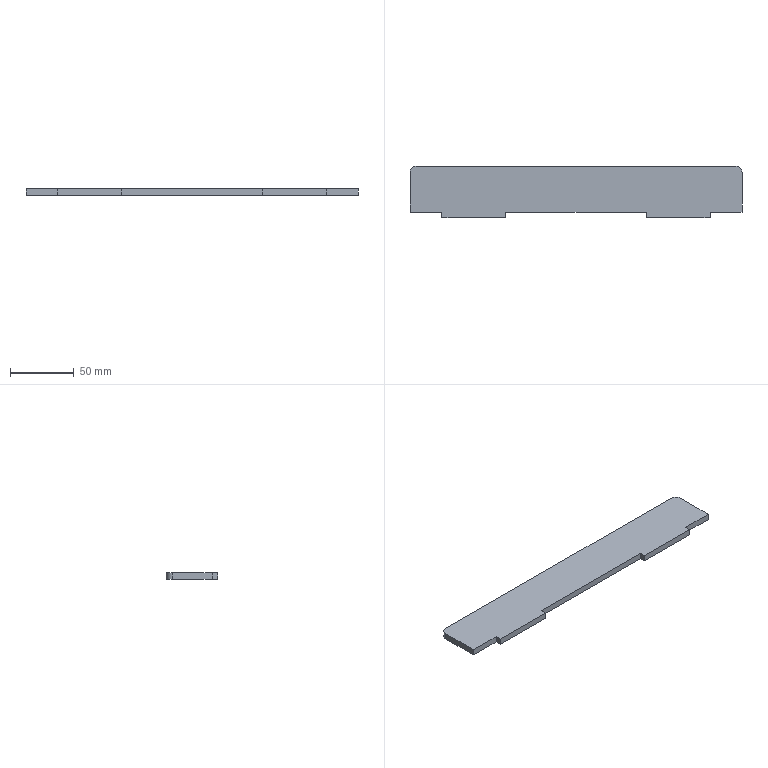Part | SolidWorks | features FlatPattern 1, SMBaseFlange 1, SheetMetal 1 | 1 solid | 16 faces | box 260 x 40.5 x 5 mm | volume 48996 mm3 | plane 14 | cylinder 2 | commonest cylinder face diameters 10 x2
STEP:
#1=CARTESIAN_POINT('',(65.526,-126.05,0.));
#2=VERTEX_POINT('',#1);
#3=CARTESIAN_POINT('',(65.526,-95.05,0.));
#4=VERTEX_POINT('',#3);
#5=CARTESIAN_POINT('',(65.526,-126.05,0.));
#6=DIRECTION('',(0.,1.,0.));
#7=VECTOR('',#6,1000.);
#8=LINE('',#5,#7);
#9=EDGE_CURVE('',#2,#4,#8,.T.);
#10=ORIENTED_EDGE('',*,*,#9,.F.);
#11=CARTESIAN_POINT('',(65.526,-126.05,-5.));
#12=VERTEX_POINT('',#11);
#13=CARTESIAN_POINT('',(65.526,-126.05,-5.));
#14=DIRECTION('',(0.,0.,1.));
#15=VECTOR('',#14,1000.);
#16=LINE('',#13,#15);
#17=EDGE_CURVE('',#12,#2,#16,.T.);
#18=ORIENTED_EDGE('',*,*,#17,.F.);
#19=CARTESIAN_POINT('',(65.526,-95.05,-5.));
#20=VERTEX_POINT('',#19);
#21=CARTESIAN_POINT('',(65.526,-126.05,-5.));
#22=DIRECTION('',(0.,1.,0.));
#23=VECTOR('',#22,1000.);
#24=LINE('',#21,#23);
#25=EDGE_CURVE('',#12,#20,#24,.T.);
#26=ORIENTED_EDGE('',*,*,#25,.T.);
#27=CARTESIAN_POINT('',(65.526,-95.05,-5.));
#28=DIRECTION('',(0.,0.,1.));
#29=VECTOR('',#28,1000.);
#30=LINE('',#27,#29);
#31=EDGE_CURVE('',#20,#4,#30,.T.);
#32=ORIENTED_EDGE('',*,*,#31,.T.);
#33=EDGE_LOOP('',(#10,#18,#26,#32));
#34=FACE_OUTER_BOUND('',#33,.T.);
#35=CARTESIAN_POINT('',(65.526,-126.05,-5.));
#36=DIRECTION('',(1.,0.,0.));
#37=DIRECTION('',(0.,0.,-1.));
#38=AXIS2_PLACEMENT_3D('',#35,#36,#37);
#39=PLANE('',#38);
#40=ADVANCED_FACE('',(#34),#39,.T.);
#41=CARTESIAN_POINT('',(40.526,-126.05,0.));
#42=VERTEX_POINT('',#41);
#43=CARTESIAN_POINT('',(65.526,-126.05,0.));
#44=DIRECTION('',(1.,0.,0.));
#45=VECTOR('',#44,1000.);
#46=LINE('',#43,#45);
#47=EDGE_CURVE('',#42,#2,#46,.T.);
#48=ORIENTED_EDGE('',*,*,#47,.F.);
#49=CARTESIAN_POINT('',(40.526,-126.05,-5.));
#50=VERTEX_POINT('',#49);
#51=CARTESIAN_POINT('',(40.526,-126.05,-5.));
#52=DIRECTION('',(0.,0.,1.));
#53=VECTOR('',#52,1000.);
#54=LINE('',#51,#53);
#55=EDGE_CURVE('',#50,#42,#54,.T.);
#56=ORIENTED_EDGE('',*,*,#55,.F.);
#57=CARTESIAN_POINT('',(65.526,-126.05,-5.));
#58=DIRECTION('',(1.,0.,0.));
#59=VECTOR('',#58,1000.);
#60=LINE('',#57,#59);
#61=EDGE_CURVE('',#50,#12,#60,.T.);
#62=ORIENTED_EDGE('',*,*,#61,.T.);
#63=ORIENTED_EDGE('',*,*,#17,.T.);
#64=EDGE_LOOP('',(#48,#56,#62,#63));
#65=FACE_OUTER_BOUND('',#64,.T.);
#66=CARTESIAN_POINT('',(65.526,-126.05,-5.));
#67=DIRECTION('',(0.,-1.,0.));
#68=DIRECTION('',(0.,0.,-1.));
#69=AXIS2_PLACEMENT_3D('',#66,#67,#68);
#70=PLANE('',#69);
#71=ADVANCED_FACE('',(#65),#70,.T.);
#72=CARTESIAN_POINT('',(40.526,-130.55,0.));
#73=VERTEX_POINT('',#72);
#74=CARTESIAN_POINT('',(40.526,-126.05,0.));
#75=DIRECTION('',(0.,1.,0.));
#76=VECTOR('',#75,1000.);
#77=LINE('',#74,#76);
#78=EDGE_CURVE('',#73,#42,#77,.T.);
#79=ORIENTED_EDGE('',*,*,#78,.F.);
#80=CARTESIAN_POINT('',(40.526,-130.55,-5.));
#81=VERTEX_POINT('',#80);
#82=CARTESIAN_POINT('',(40.526,-130.55,-5.));
#83=DIRECTION('',(0.,0.,1.));
#84=VECTOR('',#83,1000.);
#85=LINE('',#82,#84);
#86=EDGE_CURVE('',#81,#73,#85,.T.);
#87=ORIENTED_EDGE('',*,*,#86,.F.);
#88=CARTESIAN_POINT('',(40.526,-126.05,-5.));
#89=DIRECTION('',(0.,1.,0.));
#90=VECTOR('',#89,1000.);
#91=LINE('',#88,#90);
#92=EDGE_CURVE('',#81,#50,#91,.T.);
#93=ORIENTED_EDGE('',*,*,#92,.T.);
#94=ORIENTED_EDGE('',*,*,#55,.T.);
#95=EDGE_LOOP('',(#79,#87,#93,#94));
#96=FACE_OUTER_BOUND('',#95,.T.);
#97=CARTESIAN_POINT('',(40.526,-126.05,-5.));
#98=DIRECTION('',(1.,0.,0.));
#99=DIRECTION('',(0.,0.,-1.));
#100=AXIS2_PLACEMENT_3D('',#97,#98,#99);
#101=PLANE('',#100);
#102=ADVANCED_FACE('',(#96),#101,.T.);
#103=CARTESIAN_POINT('',(-9.474,-130.55,0.));
#104=VERTEX_POINT('',#103);
#105=CARTESIAN_POINT('',(40.526,-130.55,0.));
#106=DIRECTION('',(1.,0.,0.));
#107=VECTOR('',#106,1000.);
#108=LINE('',#105,#107);
#109=EDGE_CURVE('',#104,#73,#108,.T.);
#110=ORIENTED_EDGE('',*,*,#109,.F.);
#111=CARTESIAN_POINT('',(-9.474,-130.55,-5.));
#112=VERTEX_POINT('',#111);
#113=CARTESIAN_POINT('',(-9.474,-130.55,-5.));
#114=DIRECTION('',(0.,0.,1.));
#115=VECTOR('',#114,1000.);
#116=LINE('',#113,#115);
#117=EDGE_CURVE('',#112,#104,#116,.T.);
#118=ORIENTED_EDGE('',*,*,#117,.F.);
#119=CARTESIAN_POINT('',(40.526,-130.55,-5.));
#120=DIRECTION('',(1.,0.,0.));
#121=VECTOR('',#120,1000.);
#122=LINE('',#119,#121);
#123=EDGE_CURVE('',#112,#81,#122,.T.);
#124=ORIENTED_EDGE('',*,*,#123,.T.);
#125=ORIENTED_EDGE('',*,*,#86,.T.);
#126=EDGE_LOOP('',(#110,#118,#124,#125));
#127=FACE_OUTER_BOUND('',#126,.T.);
#128=CARTESIAN_POINT('',(40.526,-130.55,-5.));
#129=DIRECTION('',(0.,-1.,0.));
#130=DIRECTION('',(1.,0.,0.));
#131=AXIS2_PLACEMENT_3D('',#128,#129,#130);
#132=PLANE('',#131);
#133=ADVANCED_FACE('',(#127),#132,.T.);
#134=CARTESIAN_POINT('',(-9.474,-126.05,0.));
#135=VERTEX_POINT('',#134);
#136=CARTESIAN_POINT('',(-9.474,-130.55,0.));
#137=DIRECTION('',(0.,-1.,0.));
#138=VECTOR('',#137,1000.);
#139=LINE('',#136,#138);
#140=EDGE_CURVE('',#135,#104,#139,.T.);
#141=ORIENTED_EDGE('',*,*,#140,.F.);
#142=CARTESIAN_POINT('',(-9.474,-126.05,-5.));
#143=VERTEX_POINT('',#142);
#144=CARTESIAN_POINT('',(-9.474,-126.05,-5.));
#145=DIRECTION('',(0.,0.,1.));
#146=VECTOR('',#145,1000.);
#147=LINE('',#144,#146);
#148=EDGE_CURVE('',#143,#135,#147,.T.);
#149=ORIENTED_EDGE('',*,*,#148,.F.);
#150=CARTESIAN_POINT('',(-9.474,-130.55,-5.));
#151=DIRECTION('',(0.,-1.,0.));
#152=VECTOR('',#151,1000.);
#153=LINE('',#150,#152);
#154=EDGE_CURVE('',#143,#112,#153,.T.);
#155=ORIENTED_EDGE('',*,*,#154,.T.);
#156=ORIENTED_EDGE('',*,*,#117,.T.);
#157=EDGE_LOOP('',(#141,#149,#155,#156));
#158=FACE_OUTER_BOUND('',#157,.T.);
#159=CARTESIAN_POINT('',(-9.474,-130.55,-5.));
#160=DIRECTION('',(-1.,0.,0.));
#161=DIRECTION('',(0.,0.,1.));
#162=AXIS2_PLACEMENT_3D('',#159,#160,#161);
#163=PLANE('',#162);
#164=ADVANCED_FACE('',(#158),#163,.T.);
#165=CARTESIAN_POINT('',(-119.474,-126.05,0.));
#166=VERTEX_POINT('',#165);
#167=CARTESIAN_POINT('',(-9.474,-126.05,0.));
#168=DIRECTION('',(1.,0.,0.));
#169=VECTOR('',#168,1000.);
#170=LINE('',#167,#169);
#171=EDGE_CURVE('',#166,#135,#170,.T.);
#172=ORIENTED_EDGE('',*,*,#171,.F.);
#173=CARTESIAN_POINT('',(-119.474,-126.05,-5.));
#174=VERTEX_POINT('',#173);
#175=CARTESIAN_POINT('',(-119.474,-126.05,-5.));
#176=DIRECTION('',(0.,0.,1.));
#177=VECTOR('',#176,1000.);
#178=LINE('',#175,#177);
#179=EDGE_CURVE('',#174,#166,#178,.T.);
#180=ORIENTED_EDGE('',*,*,#179,.F.);
#181=CARTESIAN_POINT('',(-9.474,-126.05,-5.));
#182=DIRECTION('',(1.,0.,0.));
#183=VECTOR('',#182,1000.);
#184=LINE('',#181,#183);
#185=EDGE_CURVE('',#174,#143,#184,.T.);
#186=ORIENTED_EDGE('',*,*,#185,.T.);
#187=ORIENTED_EDGE('',*,*,#148,.T.);
#188=EDGE_LOOP('',(#172,#180,#186,#187));
#189=FACE_OUTER_BOUND('',#188,.T.);
#190=CARTESIAN_POINT('',(-9.474,-126.05,-5.));
#191=DIRECTION('',(0.,-1.,0.));
#192=DIRECTION('',(0.,0.,-1.));
#193=AXIS2_PLACEMENT_3D('',#190,#191,#192);
#194=PLANE('',#193);
#195=ADVANCED_FACE('',(#189),#194,.T.);
#196=CARTESIAN_POINT('',(-119.474,-130.55,0.));
#197=VERTEX_POINT('',#196);
#198=CARTESIAN_POINT('',(-119.474,-130.55,0.));
#199=DIRECTION('',(0.,1.,0.));
#200=VECTOR('',#199,1000.);
#201=LINE('',#198,#200);
#202=EDGE_CURVE('',#197,#166,#201,.T.);
#203=ORIENTED_EDGE('',*,*,#202,.F.);
#204=CARTESIAN_POINT('',(-119.474,-130.55,-5.));
#205=VERTEX_POINT('',#204);
#206=CARTESIAN_POINT('',(-119.474,-130.55,-5.));
#207=DIRECTION('',(0.,0.,1.));
#208=VECTOR('',#207,1000.);
#209=LINE('',#206,#208);
#210=EDGE_CURVE('',#205,#197,#209,.T.);
#211=ORIENTED_EDGE('',*,*,#210,.F.);
#212=CARTESIAN_POINT('',(-119.474,-130.55,-5.));
#213=DIRECTION('',(0.,1.,0.));
#214=VECTOR('',#213,1000.);
#215=LINE('',#212,#214);
#216=EDGE_CURVE('',#205,#174,#215,.T.);
#217=ORIENTED_EDGE('',*,*,#216,.T.);
#218=ORIENTED_EDGE('',*,*,#179,.T.);
#219=EDGE_LOOP('',(#203,#211,#217,#218));
#220=FACE_OUTER_BOUND('',#219,.T.);
#221=CARTESIAN_POINT('',(-119.474,-130.55,-5.));
#222=DIRECTION('',(1.,0.,0.));
#223=DIRECTION('',(0.,0.,-1.));
#224=AXIS2_PLACEMENT_3D('',#221,#222,#223);
#225=PLANE('',#224);
#226=ADVANCED_FACE('',(#220),#225,.T.);
#227=CARTESIAN_POINT('',(-169.474,-130.55,0.));
#228=VERTEX_POINT('',#227);
#229=CARTESIAN_POINT('',(-169.474,-130.55,0.));
#230=DIRECTION('',(1.,0.,0.));
#231=VECTOR('',#230,1000.);
#232=LINE('',#229,#231);
#233=EDGE_CURVE('',#228,#197,#232,.T.);
#234=ORIENTED_EDGE('',*,*,#233,.F.);
#235=CARTESIAN_POINT('',(-169.474,-130.55,-5.));
#236=VERTEX_POINT('',#235);
#237=CARTESIAN_POINT('',(-169.474,-130.55,-5.));
#238=DIRECTION('',(0.,0.,1.));
#239=VECTOR('',#238,1000.);
#240=LINE('',#237,#239);
#241=EDGE_CURVE('',#236,#228,#240,.T.);
#242=ORIENTED_EDGE('',*,*,#241,.F.);
#243=CARTESIAN_POINT('',(-169.474,-130.55,-5.));
#244=DIRECTION('',(1.,0.,0.));
#245=VECTOR('',#244,1000.);
#246=LINE('',#243,#245);
#247=EDGE_CURVE('',#236,#205,#246,.T.);
#248=ORIENTED_EDGE('',*,*,#247,.T.);
#249=ORIENTED_EDGE('',*,*,#210,.T.);
#250=EDGE_LOOP('',(#234,#242,#248,#249));
#251=FACE_OUTER_BOUND('',#250,.T.);
#252=CARTESIAN_POINT('',(-169.474,-130.55,-5.));
#253=DIRECTION('',(0.,-1.,0.));
#254=DIRECTION('',(0.,0.,-1.));
#255=AXIS2_PLACEMENT_3D('',#252,#253,#254);
#256=PLANE('',#255);
#257=ADVANCED_FACE('',(#251),#256,.T.);
#258=CARTESIAN_POINT('',(-169.474,-126.05,0.));
#259=VERTEX_POINT('',#258);
#260=CARTESIAN_POINT('',(-169.474,-126.05,0.));
#261=DIRECTION('',(0.,-1.,0.));
#262=VECTOR('',#261,1000.);
#263=LINE('',#260,#262);
#264=EDGE_CURVE('',#259,#228,#263,.T.);
#265=ORIENTED_EDGE('',*,*,#264,.F.);
#266=CARTESIAN_POINT('',(-169.474,-126.05,-5.));
#267=VERTEX_POINT('',#266);
#268=CARTESIAN_POINT('',(-169.474,-126.05,-5.));
#269=DIRECTION('',(0.,0.,1.));
#270=VECTOR('',#269,1000.);
#271=LINE('',#268,#270);
#272=EDGE_CURVE('',#267,#259,#271,.T.);
#273=ORIENTED_EDGE('',*,*,#272,.F.);
#274=CARTESIAN_POINT('',(-169.474,-126.05,-5.));
#275=DIRECTION('',(0.,-1.,0.));
#276=VECTOR('',#275,1000.);
#277=LINE('',#274,#276);
#278=EDGE_CURVE('',#267,#236,#277,.T.);
#279=ORIENTED_EDGE('',*,*,#278,.T.);
#280=ORIENTED_EDGE('',*,*,#241,.T.);
#281=EDGE_LOOP('',(#265,#273,#279,#280));
#282=FACE_OUTER_BOUND('',#281,.T.);
#283=CARTESIAN_POINT('',(-169.474,-126.05,-5.));
#284=DIRECTION('',(-1.,0.,0.));
#285=DIRECTION('',(0.,0.,1.));
#286=AXIS2_PLACEMENT_3D('',#283,#284,#285);
#287=PLANE('',#286);
#288=ADVANCED_FACE('',(#282),#287,.T.);
#289=CARTESIAN_POINT('',(-194.474,-126.05,0.));
#290=VERTEX_POINT('',#289);
#291=CARTESIAN_POINT('',(-169.474,-126.05,0.));
#292=DIRECTION('',(1.,0.,0.));
#293=VECTOR('',#292,1000.);
#294=LINE('',#291,#293);
#295=EDGE_CURVE('',#290,#259,#294,.T.);
#296=ORIENTED_EDGE('',*,*,#295,.F.);
#297=CARTESIAN_POINT('',(-194.474,-126.05,-5.));
#298=VERTEX_POINT('',#297);
#299=CARTESIAN_POINT('',(-194.474,-126.05,-5.));
#300=DIRECTION('',(0.,0.,1.));
#301=VECTOR('',#300,1000.);
#302=LINE('',#299,#301);
#303=EDGE_CURVE('',#298,#290,#302,.T.);
#304=ORIENTED_EDGE('',*,*,#303,.F.);
#305=CARTESIAN_POINT('',(-169.474,-126.05,-5.));
#306=DIRECTION('',(1.,0.,0.));
#307=VECTOR('',#306,1000.);
#308=LINE('',#305,#307);
#309=EDGE_CURVE('',#298,#267,#308,.T.);
#310=ORIENTED_EDGE('',*,*,#309,.T.);
#311=ORIENTED_EDGE('',*,*,#272,.T.);
#312=EDGE_LOOP('',(#296,#304,#310,#311));
#313=FACE_OUTER_BOUND('',#312,.T.);
#314=CARTESIAN_POINT('',(-169.474,-126.05,-5.));
#315=DIRECTION('',(0.,-1.,0.));
#316=DIRECTION('',(0.,0.,-1.));
#317=AXIS2_PLACEMENT_3D('',#314,#315,#316);
#318=PLANE('',#317);
#319=ADVANCED_FACE('',(#313),#318,.T.);
#320=CARTESIAN_POINT('',(-194.474,-95.05,0.));
#321=VERTEX_POINT('',#320);
#322=CARTESIAN_POINT('',(-194.474,-126.05,0.));
#323=DIRECTION('',(0.,-1.,0.));
#324=VECTOR('',#323,1000.);
#325=LINE('',#322,#324);
#326=EDGE_CURVE('',#321,#290,#325,.T.);
#327=ORIENTED_EDGE('',*,*,#326,.F.);
#328=CARTESIAN_POINT('',(-194.474,-95.05,-5.));
#329=VERTEX_POINT('',#328);
#330=CARTESIAN_POINT('',(-194.474,-95.05,-5.));
#331=DIRECTION('',(0.,0.,1.));
#332=VECTOR('',#331,1000.);
#333=LINE('',#330,#332);
#334=EDGE_CURVE('',#329,#321,#333,.T.);
#335=ORIENTED_EDGE('',*,*,#334,.F.);
#336=CARTESIAN_POINT('',(-194.474,-126.05,-5.));
#337=DIRECTION('',(0.,-1.,0.));
#338=VECTOR('',#337,1000.);
#339=LINE('',#336,#338);
#340=EDGE_CURVE('',#329,#298,#339,.T.);
#341=ORIENTED_EDGE('',*,*,#340,.T.);
#342=ORIENTED_EDGE('',*,*,#303,.T.);
#343=EDGE_LOOP('',(#327,#335,#341,#342));
#344=FACE_OUTER_BOUND('',#343,.T.);
#345=CARTESIAN_POINT('',(-194.474,-126.05,-5.));
#346=DIRECTION('',(-1.,0.,0.));
#347=DIRECTION('',(0.,0.,1.));
#348=AXIS2_PLACEMENT_3D('',#345,#346,#347);
#349=PLANE('',#348);
#350=ADVANCED_FACE('',(#344),#349,.T.);
#351=CARTESIAN_POINT('',(-189.474,-90.05,0.));
#352=VERTEX_POINT('',#351);
#353=CARTESIAN_POINT('',(-189.474,-95.05,0.));
#354=DIRECTION('',(0.,0.,1.));
#355=DIRECTION('',(1.,0.,0.));
#356=AXIS2_PLACEMENT_3D('',#353,#354,#355);
#357=CIRCLE('',#356,5.);
#358=EDGE_CURVE('',#352,#321,#357,.T.);
#359=ORIENTED_EDGE('',*,*,#358,.F.);
#360=CARTESIAN_POINT('',(-189.474,-90.05,-5.));
#361=VERTEX_POINT('',#360);
#362=CARTESIAN_POINT('',(-189.474,-90.05,-5.));
#363=DIRECTION('',(0.,0.,1.));
#364=VECTOR('',#363,1000.);
#365=LINE('',#362,#364);
#366=EDGE_CURVE('',#361,#352,#365,.T.);
#367=ORIENTED_EDGE('',*,*,#366,.F.);
#368=CARTESIAN_POINT('',(-189.474,-95.05,-5.));
#369=DIRECTION('',(0.,0.,1.));
#370=DIRECTION('',(1.,0.,0.));
#371=AXIS2_PLACEMENT_3D('',#368,#369,#370);
#372=CIRCLE('',#371,5.);
#373=EDGE_CURVE('',#361,#329,#372,.T.);
#374=ORIENTED_EDGE('',*,*,#373,.T.);
#375=ORIENTED_EDGE('',*,*,#334,.T.);
#376=EDGE_LOOP('',(#359,#367,#374,#375));
#377=FACE_OUTER_BOUND('',#376,.T.);
#378=CARTESIAN_POINT('',(-189.474,-95.05,-5.));
#379=DIRECTION('',(0.,0.,1.));
#380=DIRECTION('',(1.,0.,0.));
#381=AXIS2_PLACEMENT_3D('',#378,#379,#380);
#382=CYLINDRICAL_SURFACE('',#381,5.);
#383=ADVANCED_FACE('',(#377),#382,.T.);
#384=CARTESIAN_POINT('',(60.526,-90.05,0.));
#385=VERTEX_POINT('',#384);
#386=CARTESIAN_POINT('',(60.526,-90.05,0.));
#387=DIRECTION('',(-1.,0.,0.));
#388=VECTOR('',#387,1000.);
#389=LINE('',#386,#388);
#390=EDGE_CURVE('',#385,#352,#389,.T.);
#391=ORIENTED_EDGE('',*,*,#390,.F.);
#392=CARTESIAN_POINT('',(60.526,-90.05,-5.));
#393=VERTEX_POINT('',#392);
#394=CARTESIAN_POINT('',(60.526,-90.05,-5.));
#395=DIRECTION('',(0.,0.,1.));
#396=VECTOR('',#395,1000.);
#397=LINE('',#394,#396);
#398=EDGE_CURVE('',#393,#385,#397,.T.);
#399=ORIENTED_EDGE('',*,*,#398,.F.);
#400=CARTESIAN_POINT('',(60.526,-90.05,-5.));
#401=DIRECTION('',(-1.,0.,0.));
#402=VECTOR('',#401,1000.);
#403=LINE('',#400,#402);
#404=EDGE_CURVE('',#393,#361,#403,.T.);
#405=ORIENTED_EDGE('',*,*,#404,.T.);
#406=ORIENTED_EDGE('',*,*,#366,.T.);
#407=EDGE_LOOP('',(#391,#399,#405,#406));
#408=FACE_OUTER_BOUND('',#407,.T.);
#409=CARTESIAN_POINT('',(60.526,-90.05,-5.));
#410=DIRECTION('',(0.,1.,0.));
#411=DIRECTION('',(-1.,0.,0.));
#412=AXIS2_PLACEMENT_3D('',#409,#410,#411);
#413=PLANE('',#412);
#414=ADVANCED_FACE('',(#408),#413,.T.);
#415=CARTESIAN_POINT('',(60.526,-95.05,0.));
#416=DIRECTION('',(0.,0.,1.));
#417=DIRECTION('',(1.,0.,0.));
#418=AXIS2_PLACEMENT_3D('',#415,#416,#417);
#419=CIRCLE('',#418,5.);
#420=EDGE_CURVE('',#4,#385,#419,.T.);
#421=ORIENTED_EDGE('',*,*,#420,.F.);
#422=ORIENTED_EDGE('',*,*,#31,.F.);
#423=CARTESIAN_POINT('',(60.526,-95.05,-5.));
#424=DIRECTION('',(0.,0.,1.));
#425=DIRECTION('',(1.,0.,0.));
#426=AXIS2_PLACEMENT_3D('',#423,#424,#425);
#427=CIRCLE('',#426,5.);
#428=EDGE_CURVE('',#20,#393,#427,.T.);
#429=ORIENTED_EDGE('',*,*,#428,.T.);
#430=ORIENTED_EDGE('',*,*,#398,.T.);
#431=EDGE_LOOP('',(#421,#422,#429,#430));
#432=FACE_OUTER_BOUND('',#431,.T.);
#433=CARTESIAN_POINT('',(60.526,-95.05,-5.));
#434=DIRECTION('',(0.,0.,1.));
#435=DIRECTION('',(1.,0.,0.));
#436=AXIS2_PLACEMENT_3D('',#433,#434,#435);
#437=CYLINDRICAL_SURFACE('',#436,5.);
#438=ADVANCED_FACE('',(#432),#437,.T.);
#439=ORIENTED_EDGE('',*,*,#25,.F.);
#440=ORIENTED_EDGE('',*,*,#61,.F.);
#441=ORIENTED_EDGE('',*,*,#92,.F.);
#442=ORIENTED_EDGE('',*,*,#123,.F.);
#443=ORIENTED_EDGE('',*,*,#154,.F.);
#444=ORIENTED_EDGE('',*,*,#185,.F.);
#445=ORIENTED_EDGE('',*,*,#216,.F.);
#446=ORIENTED_EDGE('',*,*,#247,.F.);
#447=ORIENTED_EDGE('',*,*,#278,.F.);
#448=ORIENTED_EDGE('',*,*,#309,.F.);
#449=ORIENTED_EDGE('',*,*,#340,.F.);
#450=ORIENTED_EDGE('',*,*,#373,.F.);
#451=ORIENTED_EDGE('',*,*,#404,.F.);
#452=ORIENTED_EDGE('',*,*,#428,.F.);
#453=EDGE_LOOP('',(#439,#440,#441,#442,#443,#444,#445,#446,#447,#448,#449,#450,#451,#452));
#454=FACE_OUTER_BOUND('',#453,.T.);
#455=CARTESIAN_POINT('',(60.526,-95.05,-5.));
#456=DIRECTION('',(0.,0.,1.));
#457=DIRECTION('',(1.,0.,0.));
#458=AXIS2_PLACEMENT_3D('',#455,#456,#457);
#459=PLANE('',#458);
#460=ADVANCED_FACE('',(#454),#459,.F.);
#461=ORIENTED_EDGE('',*,*,#9,.T.);
#462=ORIENTED_EDGE('',*,*,#420,.T.);
#463=ORIENTED_EDGE('',*,*,#390,.T.);
#464=ORIENTED_EDGE('',*,*,#358,.T.);
#465=ORIENTED_EDGE('',*,*,#326,.T.);
#466=ORIENTED_EDGE('',*,*,#295,.T.);
#467=ORIENTED_EDGE('',*,*,#264,.T.);
#468=ORIENTED_EDGE('',*,*,#233,.T.);
#469=ORIENTED_EDGE('',*,*,#202,.T.);
#470=ORIENTED_EDGE('',*,*,#171,.T.);
#471=ORIENTED_EDGE('',*,*,#140,.T.);
#472=ORIENTED_EDGE('',*,*,#109,.T.);
#473=ORIENTED_EDGE('',*,*,#78,.T.);
#474=ORIENTED_EDGE('',*,*,#47,.T.);
#475=EDGE_LOOP('',(#461,#462,#463,#464,#465,#466,#467,#468,#469,#470,#471,#472,#473,#474));
#476=FACE_OUTER_BOUND('',#475,.T.);
#477=CARTESIAN_POINT('',(60.526,-95.05,0.));
#478=DIRECTION('',(0.,0.,1.));
#479=DIRECTION('',(1.,0.,0.));
#480=AXIS2_PLACEMENT_3D('',#477,#478,#479);
#481=PLANE('',#480);
#482=ADVANCED_FACE('',(#476),#481,.T.);
#483=CLOSED_SHELL('',(#40,#71,#102,#133,#164,#195,#226,#257,#288,#319,#350,#383,#414,#438,#460,#482));
#484=MANIFOLD_SOLID_BREP('',#483);
#485=CARTESIAN_POINT('',(0.,0.,0.));
#486=DIRECTION('',(0.,0.,1.));
#487=DIRECTION('',(1.,0.,0.));
#488=AXIS2_PLACEMENT_3D('',#485,#486,#487);
#489=(LENGTH_UNIT()NAMED_UNIT(*)SI_UNIT(.MILLI.,.METRE.));
#490=UNCERTAINTY_MEASURE_WITH_UNIT(LENGTH_MEASURE(0.00001),#489,'','');
#491=(NAMED_UNIT(*)PLANE_ANGLE_UNIT()SI_UNIT($,.RADIAN.));
#492=(NAMED_UNIT(*)SI_UNIT($,.STERADIAN.)SOLID_ANGLE_UNIT());
#493=(GEOMETRIC_REPRESENTATION_CONTEXT(3)GLOBAL_UNCERTAINTY_ASSIGNED_CONTEXT((#490))GLOBAL_UNIT_ASSIGNED_CONTEXT((#489,#491,#492))REPRESENTATION_CONTEXT('',''));
#494=ADVANCED_BREP_SHAPE_REPRESENTATION('',(#484,#488),#493);